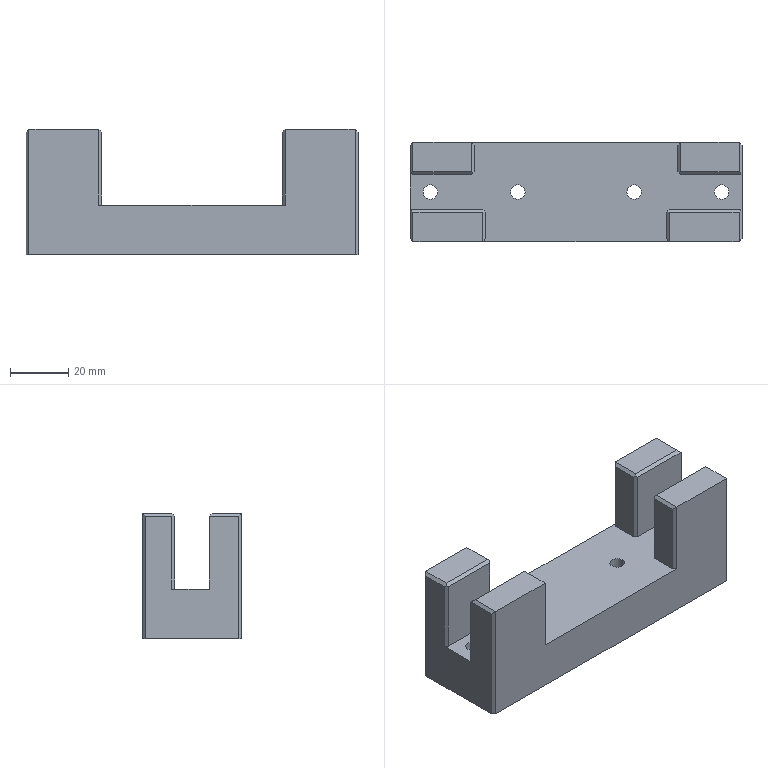Part | 1 solid | 51 faces | box 114 x 34 x 43 mm | volume 91725 mm3 | plane 43 | cylinder 8 | commonest cylinder face diameters 5 x8
STEP:
#1=CARTESIAN_POINT('',(17.5,0.,-26.));
#2=VERTEX_POINT('',#1);
#3=CARTESIAN_POINT('',(22.5,0.,-26.));
#4=VERTEX_POINT('',#3);
#5=CARTESIAN_POINT('',(20.,0.,-26.));
#6=DIRECTION('',(0.,0.,-1.));
#7=DIRECTION('',(1.,0.,0.));
#8=AXIS2_PLACEMENT_3D('',#5,#6,#7);
#9=CIRCLE('',#8,2.5);
#10=EDGE_CURVE('',#2,#4,#9,.T.);
#11=ORIENTED_EDGE('',*,*,#10,.F.);
#12=CARTESIAN_POINT('',(17.5,0.,-43.));
#13=VERTEX_POINT('',#12);
#14=CARTESIAN_POINT('',(17.5,0.,-43.));
#15=DIRECTION('',(0.,0.,-1.));
#16=VECTOR('',#15,1000.);
#17=LINE('',#14,#16);
#18=EDGE_CURVE('',#2,#13,#17,.T.);
#19=ORIENTED_EDGE('',*,*,#18,.T.);
#20=CARTESIAN_POINT('',(22.5,0.,-43.));
#21=VERTEX_POINT('',#20);
#22=CARTESIAN_POINT('',(20.,0.,-43.));
#23=DIRECTION('',(0.,0.,-1.));
#24=DIRECTION('',(1.,0.,0.));
#25=AXIS2_PLACEMENT_3D('',#22,#23,#24);
#26=CIRCLE('',#25,2.5);
#27=EDGE_CURVE('',#13,#21,#26,.T.);
#28=ORIENTED_EDGE('',*,*,#27,.T.);
#29=CARTESIAN_POINT('',(22.5,0.,-43.));
#30=DIRECTION('',(0.,0.,-1.));
#31=VECTOR('',#30,1000.);
#32=LINE('',#29,#31);
#33=EDGE_CURVE('',#4,#21,#32,.T.);
#34=ORIENTED_EDGE('',*,*,#33,.F.);
#35=EDGE_LOOP('',(#11,#19,#28,#34));
#36=FACE_BOUND('',#35,.T.);
#37=CARTESIAN_POINT('',(20.,0.,-43.));
#38=DIRECTION('',(0.,0.,-1.));
#39=DIRECTION('',(-1.,0.,0.));
#40=AXIS2_PLACEMENT_3D('',#37,#38,#39);
#41=CYLINDRICAL_SURFACE('',#40,2.5);
#42=ADVANCED_FACE('',(#36),#41,.F.);
#43=CARTESIAN_POINT('',(-22.5,0.,-26.));
#44=VERTEX_POINT('',#43);
#45=CARTESIAN_POINT('',(-17.5,0.,-26.));
#46=VERTEX_POINT('',#45);
#47=CARTESIAN_POINT('',(-20.,0.,-26.));
#48=DIRECTION('',(0.,0.,-1.));
#49=DIRECTION('',(1.,0.,0.));
#50=AXIS2_PLACEMENT_3D('',#47,#48,#49);
#51=CIRCLE('',#50,2.5);
#52=EDGE_CURVE('',#44,#46,#51,.T.);
#53=ORIENTED_EDGE('',*,*,#52,.F.);
#54=CARTESIAN_POINT('',(-22.5,0.,-43.));
#55=VERTEX_POINT('',#54);
#56=CARTESIAN_POINT('',(-22.5,0.,-43.));
#57=DIRECTION('',(0.,0.,-1.));
#58=VECTOR('',#57,1000.);
#59=LINE('',#56,#58);
#60=EDGE_CURVE('',#44,#55,#59,.T.);
#61=ORIENTED_EDGE('',*,*,#60,.T.);
#62=CARTESIAN_POINT('',(-17.5,0.,-43.));
#63=VERTEX_POINT('',#62);
#64=CARTESIAN_POINT('',(-20.,0.,-43.));
#65=DIRECTION('',(0.,0.,-1.));
#66=DIRECTION('',(1.,0.,0.));
#67=AXIS2_PLACEMENT_3D('',#64,#65,#66);
#68=CIRCLE('',#67,2.5);
#69=EDGE_CURVE('',#55,#63,#68,.T.);
#70=ORIENTED_EDGE('',*,*,#69,.T.);
#71=CARTESIAN_POINT('',(-17.5,0.,-43.));
#72=DIRECTION('',(0.,0.,-1.));
#73=VECTOR('',#72,1000.);
#74=LINE('',#71,#73);
#75=EDGE_CURVE('',#46,#63,#74,.T.);
#76=ORIENTED_EDGE('',*,*,#75,.F.);
#77=EDGE_LOOP('',(#53,#61,#70,#76));
#78=FACE_BOUND('',#77,.T.);
#79=CARTESIAN_POINT('',(-20.,0.,-43.));
#80=DIRECTION('',(0.,0.,-1.));
#81=DIRECTION('',(-1.,0.,0.));
#82=AXIS2_PLACEMENT_3D('',#79,#80,#81);
#83=CYLINDRICAL_SURFACE('',#82,2.5);
#84=ADVANCED_FACE('',(#78),#83,.F.);
#85=CARTESIAN_POINT('',(-52.5,0.,-26.));
#86=VERTEX_POINT('',#85);
#87=CARTESIAN_POINT('',(-47.5,0.,-26.));
#88=VERTEX_POINT('',#87);
#89=CARTESIAN_POINT('',(-50.,0.,-26.));
#90=DIRECTION('',(0.,0.,-1.));
#91=DIRECTION('',(1.,0.,0.));
#92=AXIS2_PLACEMENT_3D('',#89,#90,#91);
#93=CIRCLE('',#92,2.5);
#94=EDGE_CURVE('',#86,#88,#93,.T.);
#95=ORIENTED_EDGE('',*,*,#94,.F.);
#96=CARTESIAN_POINT('',(-52.5,0.,-43.));
#97=VERTEX_POINT('',#96);
#98=CARTESIAN_POINT('',(-52.5,0.,-43.));
#99=DIRECTION('',(0.,0.,-1.));
#100=VECTOR('',#99,1000.);
#101=LINE('',#98,#100);
#102=EDGE_CURVE('',#86,#97,#101,.T.);
#103=ORIENTED_EDGE('',*,*,#102,.T.);
#104=CARTESIAN_POINT('',(-47.5,0.,-43.));
#105=VERTEX_POINT('',#104);
#106=CARTESIAN_POINT('',(-50.,0.,-43.));
#107=DIRECTION('',(0.,0.,-1.));
#108=DIRECTION('',(1.,0.,0.));
#109=AXIS2_PLACEMENT_3D('',#106,#107,#108);
#110=CIRCLE('',#109,2.5);
#111=EDGE_CURVE('',#97,#105,#110,.T.);
#112=ORIENTED_EDGE('',*,*,#111,.T.);
#113=CARTESIAN_POINT('',(-47.5,0.,-43.));
#114=DIRECTION('',(0.,0.,-1.));
#115=VECTOR('',#114,1000.);
#116=LINE('',#113,#115);
#117=EDGE_CURVE('',#88,#105,#116,.T.);
#118=ORIENTED_EDGE('',*,*,#117,.F.);
#119=EDGE_LOOP('',(#95,#103,#112,#118));
#120=FACE_BOUND('',#119,.T.);
#121=CARTESIAN_POINT('',(-50.,0.,-43.));
#122=DIRECTION('',(0.,0.,-1.));
#123=DIRECTION('',(-1.,0.,0.));
#124=AXIS2_PLACEMENT_3D('',#121,#122,#123);
#125=CYLINDRICAL_SURFACE('',#124,2.5);
#126=ADVANCED_FACE('',(#120),#125,.F.);
#127=CARTESIAN_POINT('',(47.5,0.,-26.));
#128=VERTEX_POINT('',#127);
#129=CARTESIAN_POINT('',(52.5,0.,-26.));
#130=VERTEX_POINT('',#129);
#131=CARTESIAN_POINT('',(50.,0.,-26.));
#132=DIRECTION('',(0.,0.,-1.));
#133=DIRECTION('',(1.,0.,0.));
#134=AXIS2_PLACEMENT_3D('',#131,#132,#133);
#135=CIRCLE('',#134,2.5);
#136=EDGE_CURVE('',#128,#130,#135,.T.);
#137=ORIENTED_EDGE('',*,*,#136,.F.);
#138=CARTESIAN_POINT('',(47.5,0.,-43.));
#139=VERTEX_POINT('',#138);
#140=CARTESIAN_POINT('',(47.5,0.,-43.));
#141=DIRECTION('',(0.,0.,-1.));
#142=VECTOR('',#141,1000.);
#143=LINE('',#140,#142);
#144=EDGE_CURVE('',#128,#139,#143,.T.);
#145=ORIENTED_EDGE('',*,*,#144,.T.);
#146=CARTESIAN_POINT('',(52.5,0.,-43.));
#147=VERTEX_POINT('',#146);
#148=CARTESIAN_POINT('',(50.,0.,-43.));
#149=DIRECTION('',(0.,0.,-1.));
#150=DIRECTION('',(1.,0.,0.));
#151=AXIS2_PLACEMENT_3D('',#148,#149,#150);
#152=CIRCLE('',#151,2.5);
#153=EDGE_CURVE('',#139,#147,#152,.T.);
#154=ORIENTED_EDGE('',*,*,#153,.T.);
#155=CARTESIAN_POINT('',(52.5,0.,-43.));
#156=DIRECTION('',(0.,0.,-1.));
#157=VECTOR('',#156,1000.);
#158=LINE('',#155,#157);
#159=EDGE_CURVE('',#130,#147,#158,.T.);
#160=ORIENTED_EDGE('',*,*,#159,.F.);
#161=EDGE_LOOP('',(#137,#145,#154,#160));
#162=FACE_BOUND('',#161,.T.);
#163=CARTESIAN_POINT('',(50.,0.,-43.));
#164=DIRECTION('',(0.,0.,-1.));
#165=DIRECTION('',(-1.,0.,0.));
#166=AXIS2_PLACEMENT_3D('',#163,#164,#165);
#167=CYLINDRICAL_SURFACE('',#166,2.5);
#168=ADVANCED_FACE('',(#162),#167,.F.);
#169=CARTESIAN_POINT('',(36.,6.,-26.));
#170=VERTEX_POINT('',#169);
#171=CARTESIAN_POINT('',(57.,6.,-26.));
#172=VERTEX_POINT('',#171);
#173=CARTESIAN_POINT('',(57.,6.,-26.));
#174=DIRECTION('',(1.,0.,0.));
#175=VECTOR('',#174,1000.);
#176=LINE('',#173,#175);
#177=EDGE_CURVE('',#170,#172,#176,.T.);
#178=ORIENTED_EDGE('',*,*,#177,.F.);
#179=CARTESIAN_POINT('',(35.,7.,-26.));
#180=VERTEX_POINT('',#179);
#181=CARTESIAN_POINT('',(21.,21.,-26.));
#182=DIRECTION('',(-0.7071,0.7071,0.));
#183=VECTOR('',#182,1000.);
#184=LINE('',#181,#183);
#185=EDGE_CURVE('',#170,#180,#184,.T.);
#186=ORIENTED_EDGE('',*,*,#185,.T.);
#187=CARTESIAN_POINT('',(35.,16.,-26.));
#188=VERTEX_POINT('',#187);
#189=CARTESIAN_POINT('',(35.,5.,-26.));
#190=DIRECTION('',(0.,1.,0.));
#191=VECTOR('',#190,1000.);
#192=LINE('',#189,#191);
#193=EDGE_CURVE('',#180,#188,#192,.T.);
#194=ORIENTED_EDGE('',*,*,#193,.T.);
#195=CARTESIAN_POINT('',(36.,17.,-26.));
#196=VERTEX_POINT('',#195);
#197=CARTESIAN_POINT('',(9.5,-9.5,-26.));
#198=DIRECTION('',(0.7071,0.7071,0.));
#199=VECTOR('',#198,1000.);
#200=LINE('',#197,#199);
#201=EDGE_CURVE('',#188,#196,#200,.T.);
#202=ORIENTED_EDGE('',*,*,#201,.T.);
#203=CARTESIAN_POINT('',(-36.,17.,-26.));
#204=VERTEX_POINT('',#203);
#205=CARTESIAN_POINT('',(-57.,17.,-26.));
#206=DIRECTION('',(1.,0.,0.));
#207=VECTOR('',#206,1000.);
#208=LINE('',#205,#207);
#209=EDGE_CURVE('',#204,#196,#208,.T.);
#210=ORIENTED_EDGE('',*,*,#209,.F.);
#211=CARTESIAN_POINT('',(-35.,16.,-26.));
#212=VERTEX_POINT('',#211);
#213=CARTESIAN_POINT('',(-9.5,-9.5,-26.));
#214=DIRECTION('',(0.7071,-0.7071,0.));
#215=VECTOR('',#214,1000.);
#216=LINE('',#213,#215);
#217=EDGE_CURVE('',#204,#212,#216,.T.);
#218=ORIENTED_EDGE('',*,*,#217,.T.);
#219=CARTESIAN_POINT('',(-35.,7.,-26.));
#220=VERTEX_POINT('',#219);
#221=CARTESIAN_POINT('',(-35.,5.,-26.));
#222=DIRECTION('',(0.,1.,0.));
#223=VECTOR('',#222,1000.);
#224=LINE('',#221,#223);
#225=EDGE_CURVE('',#220,#212,#224,.T.);
#226=ORIENTED_EDGE('',*,*,#225,.F.);
#227=CARTESIAN_POINT('',(-36.,6.,-26.));
#228=VERTEX_POINT('',#227);
#229=CARTESIAN_POINT('',(-21.,21.,-26.));
#230=DIRECTION('',(-0.7071,-0.7071,0.));
#231=VECTOR('',#230,1000.);
#232=LINE('',#229,#231);
#233=EDGE_CURVE('',#220,#228,#232,.T.);
#234=ORIENTED_EDGE('',*,*,#233,.T.);
#235=CARTESIAN_POINT('',(-56.,6.,-26.));
#236=VERTEX_POINT('',#235);
#237=CARTESIAN_POINT('',(-57.,6.,-26.));
#238=DIRECTION('',(1.,0.,0.));
#239=VECTOR('',#238,1000.);
#240=LINE('',#237,#239);
#241=EDGE_CURVE('',#236,#228,#240,.T.);
#242=ORIENTED_EDGE('',*,*,#241,.F.);
#243=CARTESIAN_POINT('',(-57.,7.,-26.));
#244=VERTEX_POINT('',#243);
#245=CARTESIAN_POINT('',(-25.,-25.,-26.));
#246=DIRECTION('',(-0.7071,0.7071,0.));
#247=VECTOR('',#246,1000.);
#248=LINE('',#245,#247);
#249=EDGE_CURVE('',#236,#244,#248,.T.);
#250=ORIENTED_EDGE('',*,*,#249,.T.);
#251=CARTESIAN_POINT('',(-57.,-6.,-26.));
#252=VERTEX_POINT('',#251);
#253=CARTESIAN_POINT('',(-57.,-17.,-26.));
#254=DIRECTION('',(0.,1.,0.));
#255=VECTOR('',#254,1000.);
#256=LINE('',#253,#255);
#257=EDGE_CURVE('',#252,#244,#256,.T.);
#258=ORIENTED_EDGE('',*,*,#257,.F.);
#259=CARTESIAN_POINT('',(-32.,-6.,-26.));
#260=VERTEX_POINT('',#259);
#261=CARTESIAN_POINT('',(-57.,-6.,-26.));
#262=DIRECTION('',(-1.,0.,0.));
#263=VECTOR('',#262,1000.);
#264=LINE('',#261,#263);
#265=EDGE_CURVE('',#260,#252,#264,.T.);
#266=ORIENTED_EDGE('',*,*,#265,.F.);
#267=CARTESIAN_POINT('',(-31.,-7.,-26.));
#268=VERTEX_POINT('',#267);
#269=CARTESIAN_POINT('',(-19.,-19.,-26.));
#270=DIRECTION('',(0.7071,-0.7071,0.));
#271=VECTOR('',#270,1000.);
#272=LINE('',#269,#271);
#273=EDGE_CURVE('',#260,#268,#272,.T.);
#274=ORIENTED_EDGE('',*,*,#273,.T.);
#275=CARTESIAN_POINT('',(-31.,-16.,-26.));
#276=VERTEX_POINT('',#275);
#277=CARTESIAN_POINT('',(-31.,-17.,-26.));
#278=DIRECTION('',(0.,1.,0.));
#279=VECTOR('',#278,1000.);
#280=LINE('',#277,#279);
#281=EDGE_CURVE('',#276,#268,#280,.T.);
#282=ORIENTED_EDGE('',*,*,#281,.F.);
#283=CARTESIAN_POINT('',(-32.,-17.,-26.));
#284=VERTEX_POINT('',#283);
#285=CARTESIAN_POINT('',(-7.5,7.5,-26.));
#286=DIRECTION('',(-0.7071,-0.7071,0.));
#287=VECTOR('',#286,1000.);
#288=LINE('',#285,#287);
#289=EDGE_CURVE('',#276,#284,#288,.T.);
#290=ORIENTED_EDGE('',*,*,#289,.T.);
#291=CARTESIAN_POINT('',(32.,-17.,-26.));
#292=VERTEX_POINT('',#291);
#293=CARTESIAN_POINT('',(-57.,-17.,-26.));
#294=DIRECTION('',(-1.,0.,0.));
#295=VECTOR('',#294,1000.);
#296=LINE('',#293,#295);
#297=EDGE_CURVE('',#292,#284,#296,.T.);
#298=ORIENTED_EDGE('',*,*,#297,.F.);
#299=CARTESIAN_POINT('',(31.,-16.,-26.));
#300=VERTEX_POINT('',#299);
#301=CARTESIAN_POINT('',(7.5,7.5,-26.));
#302=DIRECTION('',(-0.7071,0.7071,0.));
#303=VECTOR('',#302,1000.);
#304=LINE('',#301,#303);
#305=EDGE_CURVE('',#292,#300,#304,.T.);
#306=ORIENTED_EDGE('',*,*,#305,.T.);
#307=CARTESIAN_POINT('',(31.,-7.,-26.));
#308=VERTEX_POINT('',#307);
#309=CARTESIAN_POINT('',(31.,-17.,-26.));
#310=DIRECTION('',(0.,-1.,0.));
#311=VECTOR('',#310,1000.);
#312=LINE('',#309,#311);
#313=EDGE_CURVE('',#308,#300,#312,.T.);
#314=ORIENTED_EDGE('',*,*,#313,.F.);
#315=CARTESIAN_POINT('',(32.,-6.,-26.));
#316=VERTEX_POINT('',#315);
#317=CARTESIAN_POINT('',(19.,-19.,-26.));
#318=DIRECTION('',(0.7071,0.7071,0.));
#319=VECTOR('',#318,1000.);
#320=LINE('',#317,#319);
#321=EDGE_CURVE('',#308,#316,#320,.T.);
#322=ORIENTED_EDGE('',*,*,#321,.T.);
#323=CARTESIAN_POINT('',(57.,-6.,-26.));
#324=VERTEX_POINT('',#323);
#325=CARTESIAN_POINT('',(57.,-6.,-26.));
#326=DIRECTION('',(-1.,0.,0.));
#327=VECTOR('',#326,1000.);
#328=LINE('',#325,#327);
#329=EDGE_CURVE('',#324,#316,#328,.T.);
#330=ORIENTED_EDGE('',*,*,#329,.F.);
#331=CARTESIAN_POINT('',(57.,-17.,-26.));
#332=DIRECTION('',(0.,-1.,0.));
#333=VECTOR('',#332,1000.);
#334=LINE('',#331,#333);
#335=EDGE_CURVE('',#172,#324,#334,.T.);
#336=ORIENTED_EDGE('',*,*,#335,.F.);
#337=EDGE_LOOP('',(#178,#186,#194,#202,#210,#218,#226,#234,#242,#250,#258,#266,#274,#282,#290,#298,#306,#314,#322,#330,#336));
#338=FACE_BOUND('',#337,.T.);
#339=CARTESIAN_POINT('',(20.,0.,-26.));
#340=DIRECTION('',(0.,0.,-1.));
#341=DIRECTION('',(1.,0.,0.));
#342=AXIS2_PLACEMENT_3D('',#339,#340,#341);
#343=CIRCLE('',#342,2.5);
#344=EDGE_CURVE('',#4,#2,#343,.T.);
#345=ORIENTED_EDGE('',*,*,#344,.T.);
#346=ORIENTED_EDGE('',*,*,#10,.T.);
#347=EDGE_LOOP('',(#345,#346));
#348=FACE_BOUND('',#347,.T.);
#349=CARTESIAN_POINT('',(-20.,0.,-26.));
#350=DIRECTION('',(0.,0.,-1.));
#351=DIRECTION('',(1.,0.,0.));
#352=AXIS2_PLACEMENT_3D('',#349,#350,#351);
#353=CIRCLE('',#352,2.5);
#354=EDGE_CURVE('',#46,#44,#353,.T.);
#355=ORIENTED_EDGE('',*,*,#354,.T.);
#356=ORIENTED_EDGE('',*,*,#52,.T.);
#357=EDGE_LOOP('',(#355,#356));
#358=FACE_BOUND('',#357,.T.);
#359=CARTESIAN_POINT('',(-50.,0.,-26.));
#360=DIRECTION('',(0.,0.,-1.));
#361=DIRECTION('',(1.,0.,0.));
#362=AXIS2_PLACEMENT_3D('',#359,#360,#361);
#363=CIRCLE('',#362,2.5);
#364=EDGE_CURVE('',#88,#86,#363,.T.);
#365=ORIENTED_EDGE('',*,*,#364,.T.);
#366=ORIENTED_EDGE('',*,*,#94,.T.);
#367=EDGE_LOOP('',(#365,#366));
#368=FACE_BOUND('',#367,.T.);
#369=CARTESIAN_POINT('',(50.,0.,-26.));
#370=DIRECTION('',(0.,0.,-1.));
#371=DIRECTION('',(1.,0.,0.));
#372=AXIS2_PLACEMENT_3D('',#369,#370,#371);
#373=CIRCLE('',#372,2.5);
#374=EDGE_CURVE('',#130,#128,#373,.T.);
#375=ORIENTED_EDGE('',*,*,#374,.T.);
#376=ORIENTED_EDGE('',*,*,#136,.T.);
#377=EDGE_LOOP('',(#375,#376));
#378=FACE_BOUND('',#377,.T.);
#379=CARTESIAN_POINT('',(0.,0.,-26.));
#380=DIRECTION('',(0.,0.,-1.));
#381=DIRECTION('',(-1.,0.,0.));
#382=AXIS2_PLACEMENT_3D('',#379,#380,#381);
#383=PLANE('',#382);
#384=ADVANCED_FACE('',(#338,#348,#358,#368,#378),#383,.F.);
#385=CARTESIAN_POINT('',(57.,16.,-43.));
#386=VERTEX_POINT('',#385);
#387=CARTESIAN_POINT('',(57.,-16.,-43.));
#388=VERTEX_POINT('',#387);
#389=CARTESIAN_POINT('',(57.,-17.,-43.));
#390=DIRECTION('',(0.,-1.,0.));
#391=VECTOR('',#390,1000.);
#392=LINE('',#389,#391);
#393=EDGE_CURVE('',#386,#388,#392,.T.);
#394=ORIENTED_EDGE('',*,*,#393,.F.);
#395=CARTESIAN_POINT('',(57.,16.,-1.));
#396=VERTEX_POINT('',#395);
#397=CARTESIAN_POINT('',(57.,16.,-43.));
#398=DIRECTION('',(0.,0.,1.));
#399=VECTOR('',#398,1000.);
#400=LINE('',#397,#399);
#401=EDGE_CURVE('',#386,#396,#400,.T.);
#402=ORIENTED_EDGE('',*,*,#401,.T.);
#403=CARTESIAN_POINT('',(57.,6.,-1.));
#404=VERTEX_POINT('',#403);
#405=CARTESIAN_POINT('',(57.,7.,-1.));
#406=DIRECTION('',(0.,-1.,0.));
#407=VECTOR('',#406,1000.);
#408=LINE('',#405,#407);
#409=EDGE_CURVE('',#396,#404,#408,.T.);
#410=ORIENTED_EDGE('',*,*,#409,.T.);
#411=CARTESIAN_POINT('',(57.,6.,0.));
#412=DIRECTION('',(0.,0.,-1.));
#413=VECTOR('',#412,1000.);
#414=LINE('',#411,#413);
#415=EDGE_CURVE('',#404,#172,#414,.T.);
#416=ORIENTED_EDGE('',*,*,#415,.T.);
#417=ORIENTED_EDGE('',*,*,#335,.T.);
#418=CARTESIAN_POINT('',(57.,-6.,-1.));
#419=VERTEX_POINT('',#418);
#420=CARTESIAN_POINT('',(57.,-6.,0.));
#421=DIRECTION('',(0.,0.,-1.));
#422=VECTOR('',#421,1000.);
#423=LINE('',#420,#422);
#424=EDGE_CURVE('',#419,#324,#423,.T.);
#425=ORIENTED_EDGE('',*,*,#424,.F.);
#426=CARTESIAN_POINT('',(57.,-16.,-1.));
#427=VERTEX_POINT('',#426);
#428=CARTESIAN_POINT('',(57.,-17.,-1.));
#429=DIRECTION('',(0.,-1.,0.));
#430=VECTOR('',#429,1000.);
#431=LINE('',#428,#430);
#432=EDGE_CURVE('',#419,#427,#431,.T.);
#433=ORIENTED_EDGE('',*,*,#432,.T.);
#434=CARTESIAN_POINT('',(57.,-16.,-43.));
#435=DIRECTION('',(0.,0.,-1.));
#436=VECTOR('',#435,1000.);
#437=LINE('',#434,#436);
#438=EDGE_CURVE('',#427,#388,#437,.T.);
#439=ORIENTED_EDGE('',*,*,#438,.T.);
#440=EDGE_LOOP('',(#394,#402,#410,#416,#417,#425,#433,#439));
#441=FACE_BOUND('',#440,.T.);
#442=CARTESIAN_POINT('',(57.,-17.,-43.));
#443=DIRECTION('',(-1.,0.,0.));
#444=DIRECTION('',(0.,-1.,0.));
#445=AXIS2_PLACEMENT_3D('',#442,#443,#444);
#446=PLANE('',#445);
#447=ADVANCED_FACE('',(#441),#446,.F.);
#448=CARTESIAN_POINT('',(56.,-17.,-43.));
#449=VERTEX_POINT('',#448);
#450=CARTESIAN_POINT('',(-56.,-17.,-43.));
#451=VERTEX_POINT('',#450);
#452=CARTESIAN_POINT('',(-57.,-17.,-43.));
#453=DIRECTION('',(-1.,0.,0.));
#454=VECTOR('',#453,1000.);
#455=LINE('',#452,#454);
#456=EDGE_CURVE('',#449,#451,#455,.T.);
#457=ORIENTED_EDGE('',*,*,#456,.F.);
#458=CARTESIAN_POINT('',(56.,-17.,0.));
#459=VERTEX_POINT('',#458);
#460=CARTESIAN_POINT('',(56.,-17.,-43.));
#461=DIRECTION('',(0.,0.,1.));
#462=VECTOR('',#461,1000.);
#463=LINE('',#460,#462);
#464=EDGE_CURVE('',#449,#459,#463,.T.);
#465=ORIENTED_EDGE('',*,*,#464,.T.);
#466=CARTESIAN_POINT('',(32.,-17.,0.));
#467=VERTEX_POINT('',#466);
#468=CARTESIAN_POINT('',(57.,-17.,0.));
#469=DIRECTION('',(1.,0.,0.));
#470=VECTOR('',#469,1000.);
#471=LINE('',#468,#470);
#472=EDGE_CURVE('',#467,#459,#471,.T.);
#473=ORIENTED_EDGE('',*,*,#472,.F.);
#474=CARTESIAN_POINT('',(32.,-17.,-43.));
#475=DIRECTION('',(0.,0.,-1.));
#476=VECTOR('',#475,1000.);
#477=LINE('',#474,#476);
#478=EDGE_CURVE('',#467,#292,#477,.T.);
#479=ORIENTED_EDGE('',*,*,#478,.T.);
#480=ORIENTED_EDGE('',*,*,#297,.T.);
#481=CARTESIAN_POINT('',(-32.,-17.,0.));
#482=VERTEX_POINT('',#481);
#483=CARTESIAN_POINT('',(-32.,-17.,-43.));
#484=DIRECTION('',(0.,0.,1.));
#485=VECTOR('',#484,1000.);
#486=LINE('',#483,#485);
#487=EDGE_CURVE('',#284,#482,#486,.T.);
#488=ORIENTED_EDGE('',*,*,#487,.T.);
#489=CARTESIAN_POINT('',(-56.,-17.,0.));
#490=VERTEX_POINT('',#489);
#491=CARTESIAN_POINT('',(-57.,-17.,0.));
#492=DIRECTION('',(1.,0.,0.));
#493=VECTOR('',#492,1000.);
#494=LINE('',#491,#493);
#495=EDGE_CURVE('',#490,#482,#494,.T.);
#496=ORIENTED_EDGE('',*,*,#495,.F.);
#497=CARTESIAN_POINT('',(-56.,-17.,-43.));
#498=DIRECTION('',(0.,0.,-1.));
#499=VECTOR('',#498,1000.);
#500=LINE('',#497,#499);
#501=EDGE_CURVE('',#490,#451,#500,.T.);
#502=ORIENTED_EDGE('',*,*,#501,.T.);
#503=EDGE_LOOP('',(#457,#465,#473,#479,#480,#488,#496,#502));
#504=FACE_BOUND('',#503,.T.);
#505=CARTESIAN_POINT('',(-57.,-17.,-43.));
#506=DIRECTION('',(0.,1.,0.));
#507=DIRECTION('',(0.,0.,-1.));
#508=AXIS2_PLACEMENT_3D('',#505,#506,#507);
#509=PLANE('',#508);
#510=ADVANCED_FACE('',(#504),#509,.F.);
#511=CARTESIAN_POINT('',(-57.,-16.,-43.));
#512=VERTEX_POINT('',#511);
#513=CARTESIAN_POINT('',(-57.,16.,-43.));
#514=VERTEX_POINT('',#513);
#515=CARTESIAN_POINT('',(-57.,-17.,-43.));
#516=DIRECTION('',(0.,1.,0.));
#517=VECTOR('',#516,1000.);
#518=LINE('',#515,#517);
#519=EDGE_CURVE('',#512,#514,#518,.T.);
#520=ORIENTED_EDGE('',*,*,#519,.F.);
#521=CARTESIAN_POINT('',(-57.,-16.,-1.));
#522=VERTEX_POINT('',#521);
#523=CARTESIAN_POINT('',(-57.,-16.,-43.));
#524=DIRECTION('',(0.,0.,1.));
#525=VECTOR('',#524,1000.);
#526=LINE('',#523,#525);
#527=EDGE_CURVE('',#512,#522,#526,.T.);
#528=ORIENTED_EDGE('',*,*,#527,.T.);
#529=CARTESIAN_POINT('',(-57.,-6.,-1.));
#530=VERTEX_POINT('',#529);
#531=CARTESIAN_POINT('',(-57.,-7.,-1.));
#532=DIRECTION('',(0.,1.,0.));
#533=VECTOR('',#532,1000.);
#534=LINE('',#531,#533);
#535=EDGE_CURVE('',#522,#530,#534,.T.);
#536=ORIENTED_EDGE('',*,*,#535,.T.);
#537=CARTESIAN_POINT('',(-57.,-6.,0.));
#538=DIRECTION('',(0.,0.,-1.));
#539=VECTOR('',#538,1000.);
#540=LINE('',#537,#539);
#541=EDGE_CURVE('',#530,#252,#540,.T.);
#542=ORIENTED_EDGE('',*,*,#541,.T.);
#543=ORIENTED_EDGE('',*,*,#257,.T.);
#544=CARTESIAN_POINT('',(-57.,7.,-1.));
#545=VERTEX_POINT('',#544);
#546=CARTESIAN_POINT('',(-57.,7.,-43.));
#547=DIRECTION('',(0.,0.,1.));
#548=VECTOR('',#547,1000.);
#549=LINE('',#546,#548);
#550=EDGE_CURVE('',#244,#545,#549,.T.);
#551=ORIENTED_EDGE('',*,*,#550,.T.);
#552=CARTESIAN_POINT('',(-57.,16.,-1.));
#553=VERTEX_POINT('',#552);
#554=CARTESIAN_POINT('',(-57.,17.,-1.));
#555=DIRECTION('',(0.,1.,0.));
#556=VECTOR('',#555,1000.);
#557=LINE('',#554,#556);
#558=EDGE_CURVE('',#545,#553,#557,.T.);
#559=ORIENTED_EDGE('',*,*,#558,.T.);
#560=CARTESIAN_POINT('',(-57.,16.,-43.));
#561=DIRECTION('',(0.,0.,-1.));
#562=VECTOR('',#561,1000.);
#563=LINE('',#560,#562);
#564=EDGE_CURVE('',#553,#514,#563,.T.);
#565=ORIENTED_EDGE('',*,*,#564,.T.);
#566=EDGE_LOOP('',(#520,#528,#536,#542,#543,#551,#559,#565));
#567=FACE_BOUND('',#566,.T.);
#568=CARTESIAN_POINT('',(-57.,-17.,-43.));
#569=DIRECTION('',(1.,0.,0.));
#570=DIRECTION('',(0.,1.,0.));
#571=AXIS2_PLACEMENT_3D('',#568,#569,#570);
#572=PLANE('',#571);
#573=ADVANCED_FACE('',(#567),#572,.F.);
#574=CARTESIAN_POINT('',(56.,17.,0.));
#575=VERTEX_POINT('',#574);
#576=CARTESIAN_POINT('',(36.,17.,0.));
#577=VERTEX_POINT('',#576);
#578=CARTESIAN_POINT('',(57.,17.,0.));
#579=DIRECTION('',(-1.,0.,0.));
#580=VECTOR('',#579,1000.);
#581=LINE('',#578,#580);
#582=EDGE_CURVE('',#575,#577,#581,.T.);
#583=ORIENTED_EDGE('',*,*,#582,.F.);
#584=CARTESIAN_POINT('',(56.,17.,-43.));
#585=VERTEX_POINT('',#584);
#586=CARTESIAN_POINT('',(56.,17.,-43.));
#587=DIRECTION('',(0.,0.,-1.));
#588=VECTOR('',#587,1000.);
#589=LINE('',#586,#588);
#590=EDGE_CURVE('',#575,#585,#589,.T.);
#591=ORIENTED_EDGE('',*,*,#590,.T.);
#592=CARTESIAN_POINT('',(-56.,17.,-43.));
#593=VERTEX_POINT('',#592);
#594=CARTESIAN_POINT('',(-57.,17.,-43.));
#595=DIRECTION('',(1.,0.,0.));
#596=VECTOR('',#595,1000.);
#597=LINE('',#594,#596);
#598=EDGE_CURVE('',#593,#585,#597,.T.);
#599=ORIENTED_EDGE('',*,*,#598,.F.);
#600=CARTESIAN_POINT('',(-56.,17.,0.));
#601=VERTEX_POINT('',#600);
#602=CARTESIAN_POINT('',(-56.,17.,-43.));
#603=DIRECTION('',(0.,0.,1.));
#604=VECTOR('',#603,1000.);
#605=LINE('',#602,#604);
#606=EDGE_CURVE('',#593,#601,#605,.T.);
#607=ORIENTED_EDGE('',*,*,#606,.T.);
#608=CARTESIAN_POINT('',(-36.,17.,0.));
#609=VERTEX_POINT('',#608);
#610=CARTESIAN_POINT('',(-57.,17.,0.));
#611=DIRECTION('',(-1.,0.,0.));
#612=VECTOR('',#611,1000.);
#613=LINE('',#610,#612);
#614=EDGE_CURVE('',#609,#601,#613,.T.);
#615=ORIENTED_EDGE('',*,*,#614,.F.);
#616=CARTESIAN_POINT('',(-36.,17.,-43.));
#617=DIRECTION('',(0.,0.,-1.));
#618=VECTOR('',#617,1000.);
#619=LINE('',#616,#618);
#620=EDGE_CURVE('',#609,#204,#619,.T.);
#621=ORIENTED_EDGE('',*,*,#620,.T.);
#622=ORIENTED_EDGE('',*,*,#209,.T.);
#623=CARTESIAN_POINT('',(36.,17.,-43.));
#624=DIRECTION('',(0.,0.,1.));
#625=VECTOR('',#624,1000.);
#626=LINE('',#623,#625);
#627=EDGE_CURVE('',#196,#577,#626,.T.);
#628=ORIENTED_EDGE('',*,*,#627,.T.);
#629=EDGE_LOOP('',(#583,#591,#599,#607,#615,#621,#622,#628));
#630=FACE_BOUND('',#629,.T.);
#631=CARTESIAN_POINT('',(-57.,17.,-43.));
#632=DIRECTION('',(0.,-1.,0.));
#633=DIRECTION('',(0.,0.,1.));
#634=AXIS2_PLACEMENT_3D('',#631,#632,#633);
#635=PLANE('',#634);
#636=ADVANCED_FACE('',(#630),#635,.F.);
#637=CARTESIAN_POINT('',(20.,0.,-43.));
#638=DIRECTION('',(0.,0.,-1.));
#639=DIRECTION('',(1.,0.,0.));
#640=AXIS2_PLACEMENT_3D('',#637,#638,#639);
#641=CIRCLE('',#640,2.5);
#642=EDGE_CURVE('',#21,#13,#641,.T.);
#643=ORIENTED_EDGE('',*,*,#642,.F.);
#644=ORIENTED_EDGE('',*,*,#27,.F.);
#645=EDGE_LOOP('',(#643,#644));
#646=FACE_BOUND('',#645,.T.);
#647=CARTESIAN_POINT('',(-20.,0.,-43.));
#648=DIRECTION('',(0.,0.,-1.));
#649=DIRECTION('',(1.,0.,0.));
#650=AXIS2_PLACEMENT_3D('',#647,#648,#649);
#651=CIRCLE('',#650,2.5);
#652=EDGE_CURVE('',#63,#55,#651,.T.);
#653=ORIENTED_EDGE('',*,*,#652,.F.);
#654=ORIENTED_EDGE('',*,*,#69,.F.);
#655=EDGE_LOOP('',(#653,#654));
#656=FACE_BOUND('',#655,.T.);
#657=CARTESIAN_POINT('',(-50.,0.,-43.));
#658=DIRECTION('',(0.,0.,-1.));
#659=DIRECTION('',(1.,0.,0.));
#660=AXIS2_PLACEMENT_3D('',#657,#658,#659);
#661=CIRCLE('',#660,2.5);
#662=EDGE_CURVE('',#105,#97,#661,.T.);
#663=ORIENTED_EDGE('',*,*,#662,.F.);
#664=ORIENTED_EDGE('',*,*,#111,.F.);
#665=EDGE_LOOP('',(#663,#664));
#666=FACE_BOUND('',#665,.T.);
#667=CARTESIAN_POINT('',(50.,0.,-43.));
#668=DIRECTION('',(0.,0.,-1.));
#669=DIRECTION('',(1.,0.,0.));
#670=AXIS2_PLACEMENT_3D('',#667,#668,#669);
#671=CIRCLE('',#670,2.5);
#672=EDGE_CURVE('',#147,#139,#671,.T.);
#673=ORIENTED_EDGE('',*,*,#672,.F.);
#674=ORIENTED_EDGE('',*,*,#153,.F.);
#675=EDGE_LOOP('',(#673,#674));
#676=FACE_BOUND('',#675,.T.);
#677=ORIENTED_EDGE('',*,*,#598,.T.);
#678=CARTESIAN_POINT('',(36.5,36.5,-43.));
#679=DIRECTION('',(0.7071,-0.7071,0.));
#680=VECTOR('',#679,1000.);
#681=LINE('',#678,#680);
#682=EDGE_CURVE('',#585,#386,#681,.T.);
#683=ORIENTED_EDGE('',*,*,#682,.T.);
#684=ORIENTED_EDGE('',*,*,#393,.T.);
#685=CARTESIAN_POINT('',(36.5,-36.5,-43.));
#686=DIRECTION('',(-0.7071,-0.7071,0.));
#687=VECTOR('',#686,1000.);
#688=LINE('',#685,#687);
#689=EDGE_CURVE('',#388,#449,#688,.T.);
#690=ORIENTED_EDGE('',*,*,#689,.T.);
#691=ORIENTED_EDGE('',*,*,#456,.T.);
#692=CARTESIAN_POINT('',(-36.5,-36.5,-43.));
#693=DIRECTION('',(-0.7071,0.7071,0.));
#694=VECTOR('',#693,1000.);
#695=LINE('',#692,#694);
#696=EDGE_CURVE('',#451,#512,#695,.T.);
#697=ORIENTED_EDGE('',*,*,#696,.T.);
#698=ORIENTED_EDGE('',*,*,#519,.T.);
#699=CARTESIAN_POINT('',(-36.5,36.5,-43.));
#700=DIRECTION('',(0.7071,0.7071,0.));
#701=VECTOR('',#700,1000.);
#702=LINE('',#699,#701);
#703=EDGE_CURVE('',#514,#593,#702,.T.);
#704=ORIENTED_EDGE('',*,*,#703,.T.);
#705=EDGE_LOOP('',(#677,#683,#684,#690,#691,#697,#698,#704));
#706=FACE_BOUND('',#705,.T.);
#707=CARTESIAN_POINT('',(0.,0.,-43.));
#708=DIRECTION('',(0.,0.,-1.));
#709=DIRECTION('',(-1.,0.,0.));
#710=AXIS2_PLACEMENT_3D('',#707,#708,#709);
#711=PLANE('',#710);
#712=ADVANCED_FACE('',(#646,#656,#666,#676,#706),#711,.T.);
#713=ORIENTED_EDGE('',*,*,#329,.T.);
#714=CARTESIAN_POINT('',(32.,-6.,-1.));
#715=VERTEX_POINT('',#714);
#716=CARTESIAN_POINT('',(32.,-6.,0.));
#717=DIRECTION('',(0.,0.,1.));
#718=VECTOR('',#717,1000.);
#719=LINE('',#716,#718);
#720=EDGE_CURVE('',#316,#715,#719,.T.);
#721=ORIENTED_EDGE('',*,*,#720,.T.);
#722=CARTESIAN_POINT('',(57.,-6.,-1.));
#723=DIRECTION('',(1.,0.,0.));
#724=VECTOR('',#723,1000.);
#725=LINE('',#722,#724);
#726=EDGE_CURVE('',#715,#419,#725,.T.);
#727=ORIENTED_EDGE('',*,*,#726,.T.);
#728=ORIENTED_EDGE('',*,*,#424,.T.);
#729=EDGE_LOOP('',(#713,#721,#727,#728));
#730=FACE_BOUND('',#729,.T.);
#731=CARTESIAN_POINT('',(57.,-6.,0.));
#732=DIRECTION('',(0.,-1.,0.));
#733=DIRECTION('',(1.,0.,0.));
#734=AXIS2_PLACEMENT_3D('',#731,#732,#733);
#735=PLANE('',#734);
#736=ADVANCED_FACE('',(#730),#735,.F.);
#737=ORIENTED_EDGE('',*,*,#313,.T.);
#738=CARTESIAN_POINT('',(31.,-16.,-1.));
#739=VERTEX_POINT('',#738);
#740=CARTESIAN_POINT('',(31.,-16.,0.));
#741=DIRECTION('',(0.,0.,1.));
#742=VECTOR('',#741,1000.);
#743=LINE('',#740,#742);
#744=EDGE_CURVE('',#300,#739,#743,.T.);
#745=ORIENTED_EDGE('',*,*,#744,.T.);
#746=CARTESIAN_POINT('',(31.,-7.,-1.));
#747=VERTEX_POINT('',#746);
#748=CARTESIAN_POINT('',(31.,-7.,-1.));
#749=DIRECTION('',(0.,1.,0.));
#750=VECTOR('',#749,1000.);
#751=LINE('',#748,#750);
#752=EDGE_CURVE('',#739,#747,#751,.T.);
#753=ORIENTED_EDGE('',*,*,#752,.T.);
#754=CARTESIAN_POINT('',(31.,-7.,0.));
#755=DIRECTION('',(0.,0.,-1.));
#756=VECTOR('',#755,1000.);
#757=LINE('',#754,#756);
#758=EDGE_CURVE('',#747,#308,#757,.T.);
#759=ORIENTED_EDGE('',*,*,#758,.T.);
#760=EDGE_LOOP('',(#737,#745,#753,#759));
#761=FACE_BOUND('',#760,.T.);
#762=CARTESIAN_POINT('',(31.,-17.,0.));
#763=DIRECTION('',(1.,0.,0.));
#764=DIRECTION('',(0.,1.,0.));
#765=AXIS2_PLACEMENT_3D('',#762,#763,#764);
#766=PLANE('',#765);
#767=ADVANCED_FACE('',(#761),#766,.F.);
#768=CARTESIAN_POINT('',(56.,-7.,0.));
#769=VERTEX_POINT('',#768);
#770=CARTESIAN_POINT('',(32.,-7.,0.));
#771=VERTEX_POINT('',#770);
#772=CARTESIAN_POINT('',(31.,-7.,0.));
#773=DIRECTION('',(-1.,0.,0.));
#774=VECTOR('',#773,1000.);
#775=LINE('',#772,#774);
#776=EDGE_CURVE('',#769,#771,#775,.T.);
#777=ORIENTED_EDGE('',*,*,#776,.T.);
#778=CARTESIAN_POINT('',(32.,-17.,0.));
#779=DIRECTION('',(0.,-1.,0.));
#780=VECTOR('',#779,1000.);
#781=LINE('',#778,#780);
#782=EDGE_CURVE('',#771,#467,#781,.T.);
#783=ORIENTED_EDGE('',*,*,#782,.T.);
#784=ORIENTED_EDGE('',*,*,#472,.T.);
#785=CARTESIAN_POINT('',(56.,-7.,0.));
#786=DIRECTION('',(0.,1.,0.));
#787=VECTOR('',#786,1000.);
#788=LINE('',#785,#787);
#789=EDGE_CURVE('',#459,#769,#788,.T.);
#790=ORIENTED_EDGE('',*,*,#789,.T.);
#791=EDGE_LOOP('',(#777,#783,#784,#790));
#792=FACE_BOUND('',#791,.T.);
#793=CARTESIAN_POINT('',(0.,0.,0.));
#794=DIRECTION('',(0.,0.,1.));
#795=DIRECTION('',(1.,0.,0.));
#796=AXIS2_PLACEMENT_3D('',#793,#794,#795);
#797=PLANE('',#796);
#798=ADVANCED_FACE('',(#792),#797,.T.);
#799=ORIENTED_EDGE('',*,*,#281,.T.);
#800=CARTESIAN_POINT('',(-31.,-7.,-1.));
#801=VERTEX_POINT('',#800);
#802=CARTESIAN_POINT('',(-31.,-7.,0.));
#803=DIRECTION('',(0.,0.,1.));
#804=VECTOR('',#803,1000.);
#805=LINE('',#802,#804);
#806=EDGE_CURVE('',#268,#801,#805,.T.);
#807=ORIENTED_EDGE('',*,*,#806,.T.);
#808=CARTESIAN_POINT('',(-31.,-16.,-1.));
#809=VERTEX_POINT('',#808);
#810=CARTESIAN_POINT('',(-31.,-17.,-1.));
#811=DIRECTION('',(0.,-1.,0.));
#812=VECTOR('',#811,1000.);
#813=LINE('',#810,#812);
#814=EDGE_CURVE('',#801,#809,#813,.T.);
#815=ORIENTED_EDGE('',*,*,#814,.T.);
#816=CARTESIAN_POINT('',(-31.,-16.,0.));
#817=DIRECTION('',(0.,0.,-1.));
#818=VECTOR('',#817,1000.);
#819=LINE('',#816,#818);
#820=EDGE_CURVE('',#809,#276,#819,.T.);
#821=ORIENTED_EDGE('',*,*,#820,.T.);
#822=EDGE_LOOP('',(#799,#807,#815,#821));
#823=FACE_BOUND('',#822,.T.);
#824=CARTESIAN_POINT('',(-31.,-17.,0.));
#825=DIRECTION('',(-1.,0.,0.));
#826=DIRECTION('',(0.,-1.,0.));
#827=AXIS2_PLACEMENT_3D('',#824,#825,#826);
#828=PLANE('',#827);
#829=ADVANCED_FACE('',(#823),#828,.F.);
#830=CARTESIAN_POINT('',(-32.,-6.,-1.));
#831=VERTEX_POINT('',#830);
#832=CARTESIAN_POINT('',(-31.,-6.,-1.));
#833=DIRECTION('',(1.,0.,0.));
#834=VECTOR('',#833,1000.);
#835=LINE('',#832,#834);
#836=EDGE_CURVE('',#530,#831,#835,.T.);
#837=ORIENTED_EDGE('',*,*,#836,.T.);
#838=CARTESIAN_POINT('',(-32.,-6.,0.));
#839=DIRECTION('',(0.,0.,-1.));
#840=VECTOR('',#839,1000.);
#841=LINE('',#838,#840);
#842=EDGE_CURVE('',#831,#260,#841,.T.);
#843=ORIENTED_EDGE('',*,*,#842,.T.);
#844=ORIENTED_EDGE('',*,*,#265,.T.);
#845=ORIENTED_EDGE('',*,*,#541,.F.);
#846=EDGE_LOOP('',(#837,#843,#844,#845));
#847=FACE_BOUND('',#846,.T.);
#848=CARTESIAN_POINT('',(-57.,-6.,0.));
#849=DIRECTION('',(0.,-1.,0.));
#850=DIRECTION('',(1.,0.,0.));
#851=AXIS2_PLACEMENT_3D('',#848,#849,#850);
#852=PLANE('',#851);
#853=ADVANCED_FACE('',(#847),#852,.F.);
#854=CARTESIAN_POINT('',(-32.,-7.,0.));
#855=VERTEX_POINT('',#854);
#856=CARTESIAN_POINT('',(-56.,-7.,0.));
#857=VERTEX_POINT('',#856);
#858=CARTESIAN_POINT('',(-57.,-7.,0.));
#859=DIRECTION('',(-1.,0.,0.));
#860=VECTOR('',#859,1000.);
#861=LINE('',#858,#860);
#862=EDGE_CURVE('',#855,#857,#861,.T.);
#863=ORIENTED_EDGE('',*,*,#862,.T.);
#864=CARTESIAN_POINT('',(-56.,-17.,0.));
#865=DIRECTION('',(0.,-1.,0.));
#866=VECTOR('',#865,1000.);
#867=LINE('',#864,#866);
#868=EDGE_CURVE('',#857,#490,#867,.T.);
#869=ORIENTED_EDGE('',*,*,#868,.T.);
#870=ORIENTED_EDGE('',*,*,#495,.T.);
#871=CARTESIAN_POINT('',(-32.,-7.,0.));
#872=DIRECTION('',(0.,1.,0.));
#873=VECTOR('',#872,1000.);
#874=LINE('',#871,#873);
#875=EDGE_CURVE('',#482,#855,#874,.T.);
#876=ORIENTED_EDGE('',*,*,#875,.T.);
#877=EDGE_LOOP('',(#863,#869,#870,#876));
#878=FACE_BOUND('',#877,.T.);
#879=CARTESIAN_POINT('',(0.,0.,0.));
#880=DIRECTION('',(0.,0.,1.));
#881=DIRECTION('',(1.,0.,0.));
#882=AXIS2_PLACEMENT_3D('',#879,#880,#881);
#883=PLANE('',#882);
#884=ADVANCED_FACE('',(#878),#883,.T.);
#885=CARTESIAN_POINT('',(-36.,6.,-1.));
#886=VERTEX_POINT('',#885);
#887=CARTESIAN_POINT('',(-56.,6.,-1.));
#888=VERTEX_POINT('',#887);
#889=CARTESIAN_POINT('',(-57.,6.,-1.));
#890=DIRECTION('',(-1.,0.,0.));
#891=VECTOR('',#890,1000.);
#892=LINE('',#889,#891);
#893=EDGE_CURVE('',#886,#888,#892,.T.);
#894=ORIENTED_EDGE('',*,*,#893,.T.);
#895=CARTESIAN_POINT('',(-56.,6.,0.));
#896=DIRECTION('',(0.,0.,-1.));
#897=VECTOR('',#896,1000.);
#898=LINE('',#895,#897);
#899=EDGE_CURVE('',#888,#236,#898,.T.);
#900=ORIENTED_EDGE('',*,*,#899,.T.);
#901=ORIENTED_EDGE('',*,*,#241,.T.);
#902=CARTESIAN_POINT('',(-36.,6.,0.));
#903=DIRECTION('',(0.,0.,1.));
#904=VECTOR('',#903,1000.);
#905=LINE('',#902,#904);
#906=EDGE_CURVE('',#228,#886,#905,.T.);
#907=ORIENTED_EDGE('',*,*,#906,.T.);
#908=EDGE_LOOP('',(#894,#900,#901,#907));
#909=FACE_BOUND('',#908,.T.);
#910=CARTESIAN_POINT('',(-57.,6.,0.));
#911=DIRECTION('',(0.,1.,0.));
#912=DIRECTION('',(-1.,0.,0.));
#913=AXIS2_PLACEMENT_3D('',#910,#911,#912);
#914=PLANE('',#913);
#915=ADVANCED_FACE('',(#909),#914,.F.);
#916=CARTESIAN_POINT('',(-56.,7.,0.));
#917=VERTEX_POINT('',#916);
#918=CARTESIAN_POINT('',(-36.,7.,0.));
#919=VERTEX_POINT('',#918);
#920=CARTESIAN_POINT('',(-31.,7.,0.));
#921=DIRECTION('',(1.,0.,0.));
#922=VECTOR('',#921,1000.);
#923=LINE('',#920,#922);
#924=EDGE_CURVE('',#917,#919,#923,.T.);
#925=ORIENTED_EDGE('',*,*,#924,.T.);
#926=CARTESIAN_POINT('',(-36.,17.,0.));
#927=DIRECTION('',(0.,1.,0.));
#928=VECTOR('',#927,1000.);
#929=LINE('',#926,#928);
#930=EDGE_CURVE('',#919,#609,#929,.T.);
#931=ORIENTED_EDGE('',*,*,#930,.T.);
#932=ORIENTED_EDGE('',*,*,#614,.T.);
#933=CARTESIAN_POINT('',(-56.,7.,0.));
#934=DIRECTION('',(0.,-1.,0.));
#935=VECTOR('',#934,1000.);
#936=LINE('',#933,#935);
#937=EDGE_CURVE('',#601,#917,#936,.T.);
#938=ORIENTED_EDGE('',*,*,#937,.T.);
#939=EDGE_LOOP('',(#925,#931,#932,#938));
#940=FACE_BOUND('',#939,.T.);
#941=CARTESIAN_POINT('',(0.,0.,0.));
#942=DIRECTION('',(0.,0.,1.));
#943=DIRECTION('',(1.,0.,0.));
#944=AXIS2_PLACEMENT_3D('',#941,#942,#943);
#945=PLANE('',#944);
#946=ADVANCED_FACE('',(#940),#945,.T.);
#947=CARTESIAN_POINT('',(36.,6.,-1.));
#948=VERTEX_POINT('',#947);
#949=CARTESIAN_POINT('',(31.,6.,-1.));
#950=DIRECTION('',(-1.,0.,0.));
#951=VECTOR('',#950,1000.);
#952=LINE('',#949,#951);
#953=EDGE_CURVE('',#404,#948,#952,.T.);
#954=ORIENTED_EDGE('',*,*,#953,.T.);
#955=CARTESIAN_POINT('',(36.,6.,0.));
#956=DIRECTION('',(0.,0.,-1.));
#957=VECTOR('',#956,1000.);
#958=LINE('',#955,#957);
#959=EDGE_CURVE('',#948,#170,#958,.T.);
#960=ORIENTED_EDGE('',*,*,#959,.T.);
#961=ORIENTED_EDGE('',*,*,#177,.T.);
#962=ORIENTED_EDGE('',*,*,#415,.F.);
#963=EDGE_LOOP('',(#954,#960,#961,#962));
#964=FACE_BOUND('',#963,.T.);
#965=CARTESIAN_POINT('',(57.,6.,0.));
#966=DIRECTION('',(0.,1.,0.));
#967=DIRECTION('',(-1.,0.,0.));
#968=AXIS2_PLACEMENT_3D('',#965,#966,#967);
#969=PLANE('',#968);
#970=ADVANCED_FACE('',(#964),#969,.F.);
#971=ORIENTED_EDGE('',*,*,#582,.T.);
#972=CARTESIAN_POINT('',(36.,7.,0.));
#973=VERTEX_POINT('',#972);
#974=CARTESIAN_POINT('',(36.,7.,0.));
#975=DIRECTION('',(0.,-1.,0.));
#976=VECTOR('',#975,1000.);
#977=LINE('',#974,#976);
#978=EDGE_CURVE('',#577,#973,#977,.T.);
#979=ORIENTED_EDGE('',*,*,#978,.T.);
#980=CARTESIAN_POINT('',(56.,7.,0.));
#981=VERTEX_POINT('',#980);
#982=CARTESIAN_POINT('',(57.,7.,0.));
#983=DIRECTION('',(1.,0.,0.));
#984=VECTOR('',#983,1000.);
#985=LINE('',#982,#984);
#986=EDGE_CURVE('',#973,#981,#985,.T.);
#987=ORIENTED_EDGE('',*,*,#986,.T.);
#988=CARTESIAN_POINT('',(56.,17.,0.));
#989=DIRECTION('',(0.,1.,0.));
#990=VECTOR('',#989,1000.);
#991=LINE('',#988,#990);
#992=EDGE_CURVE('',#981,#575,#991,.T.);
#993=ORIENTED_EDGE('',*,*,#992,.T.);
#994=EDGE_LOOP('',(#971,#979,#987,#993));
#995=FACE_BOUND('',#994,.T.);
#996=CARTESIAN_POINT('',(0.,0.,0.));
#997=DIRECTION('',(0.,0.,1.));
#998=DIRECTION('',(1.,0.,0.));
#999=AXIS2_PLACEMENT_3D('',#996,#997,#998);
#1000=PLANE('',#999);
#1001=ADVANCED_FACE('',(#995),#1000,.T.);
#1002=CARTESIAN_POINT('',(-56.5,6.5,-0.5));
#1003=VERTEX_POINT('',#1002);
#1004=CARTESIAN_POINT('',(-37.333,25.667,18.667));
#1005=DIRECTION('',(-0.5774,-0.5774,-0.5774));
#1006=VECTOR('',#1005,1000.);
#1007=LINE('',#1004,#1006);
#1008=EDGE_CURVE('',#917,#1003,#1007,.T.);
#1009=ORIENTED_EDGE('',*,*,#1008,.T.);
#1010=CARTESIAN_POINT('',(-38.,-12.,-19.));
#1011=DIRECTION('',(0.5774,-0.5774,-0.5774));
#1012=VECTOR('',#1011,1000.);
#1013=LINE('',#1010,#1012);
#1014=EDGE_CURVE('',#1003,#888,#1013,.T.);
#1015=ORIENTED_EDGE('',*,*,#1014,.T.);
#1016=ORIENTED_EDGE('',*,*,#893,.F.);
#1017=CARTESIAN_POINT('',(-35.5,6.5,-0.5));
#1018=VERTEX_POINT('',#1017);
#1019=CARTESIAN_POINT('',(-23.333,18.667,11.667));
#1020=DIRECTION('',(0.5774,0.5774,0.5774));
#1021=VECTOR('',#1020,1000.);
#1022=LINE('',#1019,#1021);
#1023=EDGE_CURVE('',#886,#1018,#1022,.T.);
#1024=ORIENTED_EDGE('',*,*,#1023,.T.);
#1025=CARTESIAN_POINT('',(-24.,-5.,-12.));
#1026=DIRECTION('',(-0.5774,0.5774,0.5774));
#1027=VECTOR('',#1026,1000.);
#1028=LINE('',#1025,#1027);
#1029=EDGE_CURVE('',#1018,#919,#1028,.T.);
#1030=ORIENTED_EDGE('',*,*,#1029,.T.);
#1031=ORIENTED_EDGE('',*,*,#924,.F.);
#1032=EDGE_LOOP('',(#1009,#1015,#1016,#1024,#1030,#1031));
#1033=FACE_BOUND('',#1032,.T.);
#1034=CARTESIAN_POINT('',(0.,7.,0.));
#1035=DIRECTION('',(0.,-0.7071,0.7071));
#1036=DIRECTION('',(1.,0.,0.));
#1037=AXIS2_PLACEMENT_3D('',#1034,#1035,#1036);
#1038=PLANE('',#1037);
#1039=ADVANCED_FACE('',(#1033),#1038,.T.);
#1040=CARTESIAN_POINT('',(-31.5,-6.5,-0.5));
#1041=VERTEX_POINT('',#1040);
#1042=CARTESIAN_POINT('',(-21.333,3.667,-10.667));
#1043=DIRECTION('',(0.5774,0.5774,-0.5774));
#1044=VECTOR('',#1043,1000.);
#1045=LINE('',#1042,#1044);
#1046=EDGE_CURVE('',#855,#1041,#1045,.T.);
#1047=ORIENTED_EDGE('',*,*,#1046,.T.);
#1048=CARTESIAN_POINT('',(-20.667,-17.333,10.333));
#1049=DIRECTION('',(-0.5774,0.5774,-0.5774));
#1050=VECTOR('',#1049,1000.);
#1051=LINE('',#1048,#1050);
#1052=EDGE_CURVE('',#1041,#831,#1051,.T.);
#1053=ORIENTED_EDGE('',*,*,#1052,.T.);
#1054=ORIENTED_EDGE('',*,*,#836,.F.);
#1055=CARTESIAN_POINT('',(-37.333,-25.667,18.667));
#1056=DIRECTION('',(0.5774,-0.5774,0.5774));
#1057=VECTOR('',#1056,1000.);
#1058=LINE('',#1055,#1057);
#1059=EDGE_CURVE('',#530,#857,#1058,.T.);
#1060=ORIENTED_EDGE('',*,*,#1059,.T.);
#1061=ORIENTED_EDGE('',*,*,#862,.F.);
#1062=EDGE_LOOP('',(#1047,#1053,#1054,#1060,#1061));
#1063=FACE_BOUND('',#1062,.T.);
#1064=CARTESIAN_POINT('',(0.,-7.,0.));
#1065=DIRECTION('',(0.,0.7071,0.7071));
#1066=DIRECTION('',(-1.,0.,0.));
#1067=AXIS2_PLACEMENT_3D('',#1064,#1065,#1066);
#1068=PLANE('',#1067);
#1069=ADVANCED_FACE('',(#1063),#1068,.T.);
#1070=CARTESIAN_POINT('',(35.5,6.5,-0.5));
#1071=VERTEX_POINT('',#1070);
#1072=CARTESIAN_POINT('',(24.,-5.,-12.));
#1073=DIRECTION('',(-0.5774,-0.5774,-0.5774));
#1074=VECTOR('',#1073,1000.);
#1075=LINE('',#1072,#1074);
#1076=EDGE_CURVE('',#973,#1071,#1075,.T.);
#1077=ORIENTED_EDGE('',*,*,#1076,.T.);
#1078=CARTESIAN_POINT('',(23.333,18.667,11.667));
#1079=DIRECTION('',(0.5774,-0.5774,-0.5774));
#1080=VECTOR('',#1079,1000.);
#1081=LINE('',#1078,#1080);
#1082=EDGE_CURVE('',#1071,#948,#1081,.T.);
#1083=ORIENTED_EDGE('',*,*,#1082,.T.);
#1084=ORIENTED_EDGE('',*,*,#953,.F.);
#1085=CARTESIAN_POINT('',(37.333,25.667,18.667));
#1086=DIRECTION('',(-0.5774,0.5774,0.5774));
#1087=VECTOR('',#1086,1000.);
#1088=LINE('',#1085,#1087);
#1089=EDGE_CURVE('',#404,#981,#1088,.T.);
#1090=ORIENTED_EDGE('',*,*,#1089,.T.);
#1091=ORIENTED_EDGE('',*,*,#986,.F.);
#1092=EDGE_LOOP('',(#1077,#1083,#1084,#1090,#1091));
#1093=FACE_BOUND('',#1092,.T.);
#1094=CARTESIAN_POINT('',(0.,7.,0.));
#1095=DIRECTION('',(0.,-0.7071,0.7071));
#1096=DIRECTION('',(1.,0.,0.));
#1097=AXIS2_PLACEMENT_3D('',#1094,#1095,#1096);
#1098=PLANE('',#1097);
#1099=ADVANCED_FACE('',(#1093),#1098,.T.);
#1100=ORIENTED_EDGE('',*,*,#726,.F.);
#1101=CARTESIAN_POINT('',(31.5,-6.5,-0.5));
#1102=VERTEX_POINT('',#1101);
#1103=CARTESIAN_POINT('',(20.667,-17.333,10.333));
#1104=DIRECTION('',(-0.5774,-0.5774,0.5774));
#1105=VECTOR('',#1104,1000.);
#1106=LINE('',#1103,#1105);
#1107=EDGE_CURVE('',#715,#1102,#1106,.T.);
#1108=ORIENTED_EDGE('',*,*,#1107,.T.);
#1109=CARTESIAN_POINT('',(21.333,3.667,-10.667));
#1110=DIRECTION('',(0.5774,-0.5774,0.5774));
#1111=VECTOR('',#1110,1000.);
#1112=LINE('',#1109,#1111);
#1113=EDGE_CURVE('',#1102,#771,#1112,.T.);
#1114=ORIENTED_EDGE('',*,*,#1113,.T.);
#1115=ORIENTED_EDGE('',*,*,#776,.F.);
#1116=CARTESIAN_POINT('',(37.333,-25.667,18.667));
#1117=DIRECTION('',(0.5774,0.5774,-0.5774));
#1118=VECTOR('',#1117,1000.);
#1119=LINE('',#1116,#1118);
#1120=EDGE_CURVE('',#769,#419,#1119,.T.);
#1121=ORIENTED_EDGE('',*,*,#1120,.T.);
#1122=EDGE_LOOP('',(#1100,#1108,#1114,#1115,#1121));
#1123=FACE_BOUND('',#1122,.T.);
#1124=CARTESIAN_POINT('',(0.,-7.,0.));
#1125=DIRECTION('',(0.,0.7071,0.7071));
#1126=DIRECTION('',(-1.,0.,0.));
#1127=AXIS2_PLACEMENT_3D('',#1124,#1125,#1126);
#1128=PLANE('',#1127);
#1129=ADVANCED_FACE('',(#1123),#1128,.T.);
#1130=ORIENTED_EDGE('',*,*,#937,.F.);
#1131=CARTESIAN_POINT('',(-61.667,11.333,-5.667));
#1132=DIRECTION('',(-0.5774,-0.5774,-0.5774));
#1133=VECTOR('',#1132,1000.);
#1134=LINE('',#1131,#1133);
#1135=EDGE_CURVE('',#601,#553,#1134,.T.);
#1136=ORIENTED_EDGE('',*,*,#1135,.T.);
#1137=ORIENTED_EDGE('',*,*,#558,.F.);
#1138=CARTESIAN_POINT('',(-54.,4.,2.));
#1139=DIRECTION('',(0.5774,-0.5774,0.5774));
#1140=VECTOR('',#1139,1000.);
#1141=LINE('',#1138,#1140);
#1142=EDGE_CURVE('',#545,#1003,#1141,.T.);
#1143=ORIENTED_EDGE('',*,*,#1142,.T.);
#1144=ORIENTED_EDGE('',*,*,#1008,.F.);
#1145=EDGE_LOOP('',(#1130,#1136,#1137,#1143,#1144));
#1146=FACE_BOUND('',#1145,.T.);
#1147=CARTESIAN_POINT('',(-56.,0.,0.));
#1148=DIRECTION('',(-0.7071,0.,0.7071));
#1149=DIRECTION('',(0.,-1.,0.));
#1150=AXIS2_PLACEMENT_3D('',#1147,#1148,#1149);
#1151=PLANE('',#1150);
#1152=ADVANCED_FACE('',(#1146),#1151,.T.);
#1153=ORIENTED_EDGE('',*,*,#535,.F.);
#1154=CARTESIAN_POINT('',(-61.667,-11.333,-5.667));
#1155=DIRECTION('',(0.5774,-0.5774,0.5774));
#1156=VECTOR('',#1155,1000.);
#1157=LINE('',#1154,#1156);
#1158=EDGE_CURVE('',#522,#490,#1157,.T.);
#1159=ORIENTED_EDGE('',*,*,#1158,.T.);
#1160=ORIENTED_EDGE('',*,*,#868,.F.);
#1161=ORIENTED_EDGE('',*,*,#1059,.F.);
#1162=EDGE_LOOP('',(#1153,#1159,#1160,#1161));
#1163=FACE_BOUND('',#1162,.T.);
#1164=CARTESIAN_POINT('',(-56.,0.,0.));
#1165=DIRECTION('',(-0.7071,0.,0.7071));
#1166=DIRECTION('',(0.,-1.,0.));
#1167=AXIS2_PLACEMENT_3D('',#1164,#1165,#1166);
#1168=PLANE('',#1167);
#1169=ADVANCED_FACE('',(#1163),#1168,.T.);
#1170=ORIENTED_EDGE('',*,*,#814,.F.);
#1171=CARTESIAN_POINT('',(-34.,-4.,2.));
#1172=DIRECTION('',(-0.5774,0.5774,0.5774));
#1173=VECTOR('',#1172,1000.);
#1174=LINE('',#1171,#1173);
#1175=EDGE_CURVE('',#801,#1041,#1174,.T.);
#1176=ORIENTED_EDGE('',*,*,#1175,.T.);
#1177=ORIENTED_EDGE('',*,*,#1046,.F.);
#1178=ORIENTED_EDGE('',*,*,#875,.F.);
#1179=CARTESIAN_POINT('',(-26.333,-11.333,-5.667));
#1180=DIRECTION('',(0.5774,0.5774,-0.5774));
#1181=VECTOR('',#1180,1000.);
#1182=LINE('',#1179,#1181);
#1183=EDGE_CURVE('',#482,#809,#1182,.T.);
#1184=ORIENTED_EDGE('',*,*,#1183,.T.);
#1185=EDGE_LOOP('',(#1170,#1176,#1177,#1178,#1184));
#1186=FACE_BOUND('',#1185,.T.);
#1187=CARTESIAN_POINT('',(-32.,0.,0.));
#1188=DIRECTION('',(0.7071,0.,0.7071));
#1189=DIRECTION('',(0.,1.,0.));
#1190=AXIS2_PLACEMENT_3D('',#1187,#1188,#1189);
#1191=PLANE('',#1190);
#1192=ADVANCED_FACE('',(#1186),#1191,.T.);
#1193=ORIENTED_EDGE('',*,*,#409,.F.);
#1194=CARTESIAN_POINT('',(61.667,11.333,-5.667));
#1195=DIRECTION('',(-0.5774,0.5774,0.5774));
#1196=VECTOR('',#1195,1000.);
#1197=LINE('',#1194,#1196);
#1198=EDGE_CURVE('',#396,#575,#1197,.T.);
#1199=ORIENTED_EDGE('',*,*,#1198,.T.);
#1200=ORIENTED_EDGE('',*,*,#992,.F.);
#1201=ORIENTED_EDGE('',*,*,#1089,.F.);
#1202=EDGE_LOOP('',(#1193,#1199,#1200,#1201));
#1203=FACE_BOUND('',#1202,.T.);
#1204=CARTESIAN_POINT('',(56.,0.,0.));
#1205=DIRECTION('',(0.7071,0.,0.7071));
#1206=DIRECTION('',(0.,1.,0.));
#1207=AXIS2_PLACEMENT_3D('',#1204,#1205,#1206);
#1208=PLANE('',#1207);
#1209=ADVANCED_FACE('',(#1203),#1208,.T.);
#1210=ORIENTED_EDGE('',*,*,#752,.F.);
#1211=CARTESIAN_POINT('',(26.333,-11.333,-5.667));
#1212=DIRECTION('',(0.5774,-0.5774,0.5774));
#1213=VECTOR('',#1212,1000.);
#1214=LINE('',#1211,#1213);
#1215=EDGE_CURVE('',#739,#467,#1214,.T.);
#1216=ORIENTED_EDGE('',*,*,#1215,.T.);
#1217=ORIENTED_EDGE('',*,*,#782,.F.);
#1218=ORIENTED_EDGE('',*,*,#1113,.F.);
#1219=CARTESIAN_POINT('',(34.,-4.,2.));
#1220=DIRECTION('',(-0.5774,-0.5774,-0.5774));
#1221=VECTOR('',#1220,1000.);
#1222=LINE('',#1219,#1221);
#1223=EDGE_CURVE('',#1102,#747,#1222,.T.);
#1224=ORIENTED_EDGE('',*,*,#1223,.T.);
#1225=EDGE_LOOP('',(#1210,#1216,#1217,#1218,#1224));
#1226=FACE_BOUND('',#1225,.T.);
#1227=CARTESIAN_POINT('',(32.,0.,0.));
#1228=DIRECTION('',(-0.7071,0.,0.7071));
#1229=DIRECTION('',(0.,-1.,0.));
#1230=AXIS2_PLACEMENT_3D('',#1227,#1228,#1229);
#1231=PLANE('',#1230);
#1232=ADVANCED_FACE('',(#1226),#1231,.T.);
#1233=ORIENTED_EDGE('',*,*,#789,.F.);
#1234=CARTESIAN_POINT('',(61.667,-11.333,-5.667));
#1235=DIRECTION('',(0.5774,0.5774,-0.5774));
#1236=VECTOR('',#1235,1000.);
#1237=LINE('',#1234,#1236);
#1238=EDGE_CURVE('',#459,#427,#1237,.T.);
#1239=ORIENTED_EDGE('',*,*,#1238,.T.);
#1240=ORIENTED_EDGE('',*,*,#432,.F.);
#1241=ORIENTED_EDGE('',*,*,#1120,.F.);
#1242=EDGE_LOOP('',(#1233,#1239,#1240,#1241));
#1243=FACE_BOUND('',#1242,.T.);
#1244=CARTESIAN_POINT('',(56.,0.,0.));
#1245=DIRECTION('',(0.7071,0.,0.7071));
#1246=DIRECTION('',(0.,1.,0.));
#1247=AXIS2_PLACEMENT_3D('',#1244,#1245,#1246);
#1248=PLANE('',#1247);
#1249=ADVANCED_FACE('',(#1243),#1248,.T.);
#1250=ORIENTED_EDGE('',*,*,#144,.F.);
#1251=ORIENTED_EDGE('',*,*,#374,.F.);
#1252=ORIENTED_EDGE('',*,*,#159,.T.);
#1253=ORIENTED_EDGE('',*,*,#672,.T.);
#1254=EDGE_LOOP('',(#1250,#1251,#1252,#1253));
#1255=FACE_BOUND('',#1254,.T.);
#1256=CARTESIAN_POINT('',(50.,0.,-43.));
#1257=DIRECTION('',(0.,0.,-1.));
#1258=DIRECTION('',(-1.,0.,0.));
#1259=AXIS2_PLACEMENT_3D('',#1256,#1257,#1258);
#1260=CYLINDRICAL_SURFACE('',#1259,2.5);
#1261=ADVANCED_FACE('',(#1255),#1260,.F.);
#1262=ORIENTED_EDGE('',*,*,#102,.F.);
#1263=ORIENTED_EDGE('',*,*,#364,.F.);
#1264=ORIENTED_EDGE('',*,*,#117,.T.);
#1265=ORIENTED_EDGE('',*,*,#662,.T.);
#1266=EDGE_LOOP('',(#1262,#1263,#1264,#1265));
#1267=FACE_BOUND('',#1266,.T.);
#1268=CARTESIAN_POINT('',(-50.,0.,-43.));
#1269=DIRECTION('',(0.,0.,-1.));
#1270=DIRECTION('',(-1.,0.,0.));
#1271=AXIS2_PLACEMENT_3D('',#1268,#1269,#1270);
#1272=CYLINDRICAL_SURFACE('',#1271,2.5);
#1273=ADVANCED_FACE('',(#1267),#1272,.F.);
#1274=ORIENTED_EDGE('',*,*,#60,.F.);
#1275=ORIENTED_EDGE('',*,*,#354,.F.);
#1276=ORIENTED_EDGE('',*,*,#75,.T.);
#1277=ORIENTED_EDGE('',*,*,#652,.T.);
#1278=EDGE_LOOP('',(#1274,#1275,#1276,#1277));
#1279=FACE_BOUND('',#1278,.T.);
#1280=CARTESIAN_POINT('',(-20.,0.,-43.));
#1281=DIRECTION('',(0.,0.,-1.));
#1282=DIRECTION('',(-1.,0.,0.));
#1283=AXIS2_PLACEMENT_3D('',#1280,#1281,#1282);
#1284=CYLINDRICAL_SURFACE('',#1283,2.5);
#1285=ADVANCED_FACE('',(#1279),#1284,.F.);
#1286=ORIENTED_EDGE('',*,*,#18,.F.);
#1287=ORIENTED_EDGE('',*,*,#344,.F.);
#1288=ORIENTED_EDGE('',*,*,#33,.T.);
#1289=ORIENTED_EDGE('',*,*,#642,.T.);
#1290=EDGE_LOOP('',(#1286,#1287,#1288,#1289));
#1291=FACE_BOUND('',#1290,.T.);
#1292=CARTESIAN_POINT('',(20.,0.,-43.));
#1293=DIRECTION('',(0.,0.,-1.));
#1294=DIRECTION('',(-1.,0.,0.));
#1295=AXIS2_PLACEMENT_3D('',#1292,#1293,#1294);
#1296=CYLINDRICAL_SURFACE('',#1295,2.5);
#1297=ADVANCED_FACE('',(#1291),#1296,.F.);
#1298=ORIENTED_EDGE('',*,*,#225,.T.);
#1299=CARTESIAN_POINT('',(-35.,16.,-1.));
#1300=VERTEX_POINT('',#1299);
#1301=CARTESIAN_POINT('',(-35.,16.,-26.));
#1302=DIRECTION('',(0.,0.,1.));
#1303=VECTOR('',#1302,1000.);
#1304=LINE('',#1301,#1303);
#1305=EDGE_CURVE('',#212,#1300,#1304,.T.);
#1306=ORIENTED_EDGE('',*,*,#1305,.T.);
#1307=CARTESIAN_POINT('',(-35.,7.,-1.));
#1308=VERTEX_POINT('',#1307);
#1309=CARTESIAN_POINT('',(-35.,7.,-1.));
#1310=DIRECTION('',(0.,-1.,0.));
#1311=VECTOR('',#1310,1000.);
#1312=LINE('',#1309,#1311);
#1313=EDGE_CURVE('',#1300,#1308,#1312,.T.);
#1314=ORIENTED_EDGE('',*,*,#1313,.T.);
#1315=CARTESIAN_POINT('',(-35.,7.,-26.));
#1316=DIRECTION('',(0.,0.,-1.));
#1317=VECTOR('',#1316,1000.);
#1318=LINE('',#1315,#1317);
#1319=EDGE_CURVE('',#1308,#220,#1318,.T.);
#1320=ORIENTED_EDGE('',*,*,#1319,.T.);
#1321=EDGE_LOOP('',(#1298,#1306,#1314,#1320));
#1322=FACE_BOUND('',#1321,.T.);
#1323=CARTESIAN_POINT('',(-35.,5.,-26.));
#1324=DIRECTION('',(-1.,0.,0.));
#1325=DIRECTION('',(0.,0.,1.));
#1326=AXIS2_PLACEMENT_3D('',#1323,#1324,#1325);
#1327=PLANE('',#1326);
#1328=ADVANCED_FACE('',(#1322),#1327,.F.);
#1329=CARTESIAN_POINT('',(35.,7.,-1.));
#1330=VERTEX_POINT('',#1329);
#1331=CARTESIAN_POINT('',(35.,16.,-1.));
#1332=VERTEX_POINT('',#1331);
#1333=CARTESIAN_POINT('',(35.,17.,-1.));
#1334=DIRECTION('',(0.,1.,0.));
#1335=VECTOR('',#1334,1000.);
#1336=LINE('',#1333,#1335);
#1337=EDGE_CURVE('',#1330,#1332,#1336,.T.);
#1338=ORIENTED_EDGE('',*,*,#1337,.T.);
#1339=CARTESIAN_POINT('',(35.,16.,-26.));
#1340=DIRECTION('',(0.,0.,-1.));
#1341=VECTOR('',#1340,1000.);
#1342=LINE('',#1339,#1341);
#1343=EDGE_CURVE('',#1332,#188,#1342,.T.);
#1344=ORIENTED_EDGE('',*,*,#1343,.T.);
#1345=ORIENTED_EDGE('',*,*,#193,.F.);
#1346=CARTESIAN_POINT('',(35.,7.,-26.));
#1347=DIRECTION('',(0.,0.,1.));
#1348=VECTOR('',#1347,1000.);
#1349=LINE('',#1346,#1348);
#1350=EDGE_CURVE('',#180,#1330,#1349,.T.);
#1351=ORIENTED_EDGE('',*,*,#1350,.T.);
#1352=EDGE_LOOP('',(#1338,#1344,#1345,#1351));
#1353=FACE_BOUND('',#1352,.T.);
#1354=CARTESIAN_POINT('',(35.,5.,-26.));
#1355=DIRECTION('',(1.,0.,0.));
#1356=DIRECTION('',(0.,0.,-1.));
#1357=AXIS2_PLACEMENT_3D('',#1354,#1355,#1356);
#1358=PLANE('',#1357);
#1359=ADVANCED_FACE('',(#1353),#1358,.F.);
#1360=ORIENTED_EDGE('',*,*,#978,.F.);
#1361=CARTESIAN_POINT('',(31.333,12.333,-4.667));
#1362=DIRECTION('',(-0.5774,-0.5774,-0.5774));
#1363=VECTOR('',#1362,1000.);
#1364=LINE('',#1361,#1363);
#1365=EDGE_CURVE('',#577,#1332,#1364,.T.);
#1366=ORIENTED_EDGE('',*,*,#1365,.T.);
#1367=ORIENTED_EDGE('',*,*,#1337,.F.);
#1368=CARTESIAN_POINT('',(35.667,6.333,-0.3333));
#1369=DIRECTION('',(0.5774,-0.5774,0.5774));
#1370=VECTOR('',#1369,1000.);
#1371=LINE('',#1368,#1370);
#1372=EDGE_CURVE('',#1330,#1071,#1371,.T.);
#1373=ORIENTED_EDGE('',*,*,#1372,.T.);
#1374=ORIENTED_EDGE('',*,*,#1076,.F.);
#1375=EDGE_LOOP('',(#1360,#1366,#1367,#1373,#1374));
#1376=FACE_BOUND('',#1375,.T.);
#1377=CARTESIAN_POINT('',(35.,5.,-1.));
#1378=DIRECTION('',(-0.7071,0.,0.7071));
#1379=DIRECTION('',(0.,1.,0.));
#1380=AXIS2_PLACEMENT_3D('',#1377,#1378,#1379);
#1381=PLANE('',#1380);
#1382=ADVANCED_FACE('',(#1376),#1381,.T.);
#1383=ORIENTED_EDGE('',*,*,#1313,.F.);
#1384=CARTESIAN_POINT('',(-30.333,11.333,-5.667));
#1385=DIRECTION('',(-0.5774,0.5774,0.5774));
#1386=VECTOR('',#1385,1000.);
#1387=LINE('',#1384,#1386);
#1388=EDGE_CURVE('',#1300,#609,#1387,.T.);
#1389=ORIENTED_EDGE('',*,*,#1388,.T.);
#1390=ORIENTED_EDGE('',*,*,#930,.F.);
#1391=ORIENTED_EDGE('',*,*,#1029,.F.);
#1392=CARTESIAN_POINT('',(-38.,4.,2.));
#1393=DIRECTION('',(0.5774,0.5774,-0.5774));
#1394=VECTOR('',#1393,1000.);
#1395=LINE('',#1392,#1394);
#1396=EDGE_CURVE('',#1018,#1308,#1395,.T.);
#1397=ORIENTED_EDGE('',*,*,#1396,.T.);
#1398=EDGE_LOOP('',(#1383,#1389,#1390,#1391,#1397));
#1399=FACE_BOUND('',#1398,.T.);
#1400=CARTESIAN_POINT('',(-36.,0.,0.));
#1401=DIRECTION('',(0.7071,0.,0.7071));
#1402=DIRECTION('',(0.,1.,0.));
#1403=AXIS2_PLACEMENT_3D('',#1400,#1401,#1402);
#1404=PLANE('',#1403);
#1405=ADVANCED_FACE('',(#1399),#1404,.T.);
#1406=ORIENTED_EDGE('',*,*,#682,.F.);
#1407=ORIENTED_EDGE('',*,*,#590,.F.);
#1408=ORIENTED_EDGE('',*,*,#1198,.F.);
#1409=ORIENTED_EDGE('',*,*,#401,.F.);
#1410=EDGE_LOOP('',(#1406,#1407,#1408,#1409));
#1411=FACE_BOUND('',#1410,.T.);
#1412=CARTESIAN_POINT('',(57.,16.,-43.));
#1413=DIRECTION('',(-0.7071,-0.7071,0.));
#1414=DIRECTION('',(0.,0.,-1.));
#1415=AXIS2_PLACEMENT_3D('',#1412,#1413,#1414);
#1416=PLANE('',#1415);
#1417=ADVANCED_FACE('',(#1411),#1416,.F.);
#1418=ORIENTED_EDGE('',*,*,#689,.F.);
#1419=ORIENTED_EDGE('',*,*,#438,.F.);
#1420=ORIENTED_EDGE('',*,*,#1238,.F.);
#1421=ORIENTED_EDGE('',*,*,#464,.F.);
#1422=EDGE_LOOP('',(#1418,#1419,#1420,#1421));
#1423=FACE_BOUND('',#1422,.T.);
#1424=CARTESIAN_POINT('',(56.,-17.,-43.));
#1425=DIRECTION('',(-0.7071,0.7071,0.));
#1426=DIRECTION('',(0.,0.,-1.));
#1427=AXIS2_PLACEMENT_3D('',#1424,#1425,#1426);
#1428=PLANE('',#1427);
#1429=ADVANCED_FACE('',(#1423),#1428,.F.);
#1430=ORIENTED_EDGE('',*,*,#1215,.F.);
#1431=ORIENTED_EDGE('',*,*,#744,.F.);
#1432=ORIENTED_EDGE('',*,*,#305,.F.);
#1433=ORIENTED_EDGE('',*,*,#478,.F.);
#1434=EDGE_LOOP('',(#1430,#1431,#1432,#1433));
#1435=FACE_BOUND('',#1434,.T.);
#1436=CARTESIAN_POINT('',(32.,-17.,-43.));
#1437=DIRECTION('',(0.7071,0.7071,0.));
#1438=DIRECTION('',(0.,0.,1.));
#1439=AXIS2_PLACEMENT_3D('',#1436,#1437,#1438);
#1440=PLANE('',#1439);
#1441=ADVANCED_FACE('',(#1435),#1440,.F.);
#1442=ORIENTED_EDGE('',*,*,#1107,.F.);
#1443=ORIENTED_EDGE('',*,*,#720,.F.);
#1444=ORIENTED_EDGE('',*,*,#321,.F.);
#1445=ORIENTED_EDGE('',*,*,#758,.F.);
#1446=ORIENTED_EDGE('',*,*,#1223,.F.);
#1447=EDGE_LOOP('',(#1442,#1443,#1444,#1445,#1446));
#1448=FACE_BOUND('',#1447,.T.);
#1449=CARTESIAN_POINT('',(31.,-7.,0.));
#1450=DIRECTION('',(0.7071,-0.7071,0.));
#1451=DIRECTION('',(0.,0.,1.));
#1452=AXIS2_PLACEMENT_3D('',#1449,#1450,#1451);
#1453=PLANE('',#1452);
#1454=ADVANCED_FACE('',(#1448),#1453,.F.);
#1455=ORIENTED_EDGE('',*,*,#1365,.F.);
#1456=ORIENTED_EDGE('',*,*,#627,.F.);
#1457=ORIENTED_EDGE('',*,*,#201,.F.);
#1458=ORIENTED_EDGE('',*,*,#1343,.F.);
#1459=EDGE_LOOP('',(#1455,#1456,#1457,#1458));
#1460=FACE_BOUND('',#1459,.T.);
#1461=CARTESIAN_POINT('',(35.,16.,-26.));
#1462=DIRECTION('',(0.7071,-0.7071,0.));
#1463=DIRECTION('',(0.,0.,1.));
#1464=AXIS2_PLACEMENT_3D('',#1461,#1462,#1463);
#1465=PLANE('',#1464);
#1466=ADVANCED_FACE('',(#1460),#1465,.F.);
#1467=ORIENTED_EDGE('',*,*,#1372,.F.);
#1468=ORIENTED_EDGE('',*,*,#1350,.F.);
#1469=ORIENTED_EDGE('',*,*,#185,.F.);
#1470=ORIENTED_EDGE('',*,*,#959,.F.);
#1471=ORIENTED_EDGE('',*,*,#1082,.F.);
#1472=EDGE_LOOP('',(#1467,#1468,#1469,#1470,#1471));
#1473=FACE_BOUND('',#1472,.T.);
#1474=CARTESIAN_POINT('',(36.,6.,0.));
#1475=DIRECTION('',(0.7071,0.7071,0.));
#1476=DIRECTION('',(0.,0.,1.));
#1477=AXIS2_PLACEMENT_3D('',#1474,#1475,#1476);
#1478=PLANE('',#1477);
#1479=ADVANCED_FACE('',(#1473),#1478,.F.);
#1480=ORIENTED_EDGE('',*,*,#696,.F.);
#1481=ORIENTED_EDGE('',*,*,#501,.F.);
#1482=ORIENTED_EDGE('',*,*,#1158,.F.);
#1483=ORIENTED_EDGE('',*,*,#527,.F.);
#1484=EDGE_LOOP('',(#1480,#1481,#1482,#1483));
#1485=FACE_BOUND('',#1484,.T.);
#1486=CARTESIAN_POINT('',(-57.,-16.,-43.));
#1487=DIRECTION('',(0.7071,0.7071,0.));
#1488=DIRECTION('',(0.,0.,-1.));
#1489=AXIS2_PLACEMENT_3D('',#1486,#1487,#1488);
#1490=PLANE('',#1489);
#1491=ADVANCED_FACE('',(#1485),#1490,.F.);
#1492=ORIENTED_EDGE('',*,*,#703,.F.);
#1493=ORIENTED_EDGE('',*,*,#564,.F.);
#1494=ORIENTED_EDGE('',*,*,#1135,.F.);
#1495=ORIENTED_EDGE('',*,*,#606,.F.);
#1496=EDGE_LOOP('',(#1492,#1493,#1494,#1495));
#1497=FACE_BOUND('',#1496,.T.);
#1498=CARTESIAN_POINT('',(-56.,17.,-43.));
#1499=DIRECTION('',(0.7071,-0.7071,0.));
#1500=DIRECTION('',(0.,0.,-1.));
#1501=AXIS2_PLACEMENT_3D('',#1498,#1499,#1500);
#1502=PLANE('',#1501);
#1503=ADVANCED_FACE('',(#1497),#1502,.F.);
#1504=ORIENTED_EDGE('',*,*,#1142,.F.);
#1505=ORIENTED_EDGE('',*,*,#550,.F.);
#1506=ORIENTED_EDGE('',*,*,#249,.F.);
#1507=ORIENTED_EDGE('',*,*,#899,.F.);
#1508=ORIENTED_EDGE('',*,*,#1014,.F.);
#1509=EDGE_LOOP('',(#1504,#1505,#1506,#1507,#1508));
#1510=FACE_BOUND('',#1509,.T.);
#1511=CARTESIAN_POINT('',(-56.,6.,0.));
#1512=DIRECTION('',(0.7071,0.7071,0.));
#1513=DIRECTION('',(0.,0.,1.));
#1514=AXIS2_PLACEMENT_3D('',#1511,#1512,#1513);
#1515=PLANE('',#1514);
#1516=ADVANCED_FACE('',(#1510),#1515,.F.);
#1517=ORIENTED_EDGE('',*,*,#217,.F.);
#1518=ORIENTED_EDGE('',*,*,#620,.F.);
#1519=ORIENTED_EDGE('',*,*,#1388,.F.);
#1520=ORIENTED_EDGE('',*,*,#1305,.F.);
#1521=EDGE_LOOP('',(#1517,#1518,#1519,#1520));
#1522=FACE_BOUND('',#1521,.T.);
#1523=CARTESIAN_POINT('',(-35.,16.,-26.));
#1524=DIRECTION('',(-0.7071,-0.7071,0.));
#1525=DIRECTION('',(0.,0.,-1.));
#1526=AXIS2_PLACEMENT_3D('',#1523,#1524,#1525);
#1527=PLANE('',#1526);
#1528=ADVANCED_FACE('',(#1522),#1527,.F.);
#1529=ORIENTED_EDGE('',*,*,#233,.F.);
#1530=ORIENTED_EDGE('',*,*,#1319,.F.);
#1531=ORIENTED_EDGE('',*,*,#1396,.F.);
#1532=ORIENTED_EDGE('',*,*,#1023,.F.);
#1533=ORIENTED_EDGE('',*,*,#906,.F.);
#1534=EDGE_LOOP('',(#1529,#1530,#1531,#1532,#1533));
#1535=FACE_BOUND('',#1534,.T.);
#1536=CARTESIAN_POINT('',(-36.,6.,0.));
#1537=DIRECTION('',(-0.7071,0.7071,0.));
#1538=DIRECTION('',(0.,0.,-1.));
#1539=AXIS2_PLACEMENT_3D('',#1536,#1537,#1538);
#1540=PLANE('',#1539);
#1541=ADVANCED_FACE('',(#1535),#1540,.F.);
#1542=ORIENTED_EDGE('',*,*,#1175,.F.);
#1543=ORIENTED_EDGE('',*,*,#806,.F.);
#1544=ORIENTED_EDGE('',*,*,#273,.F.);
#1545=ORIENTED_EDGE('',*,*,#842,.F.);
#1546=ORIENTED_EDGE('',*,*,#1052,.F.);
#1547=EDGE_LOOP('',(#1542,#1543,#1544,#1545,#1546));
#1548=FACE_BOUND('',#1547,.T.);
#1549=CARTESIAN_POINT('',(-32.,-6.,0.));
#1550=DIRECTION('',(-0.7071,-0.7071,0.));
#1551=DIRECTION('',(0.,0.,1.));
#1552=AXIS2_PLACEMENT_3D('',#1549,#1550,#1551);
#1553=PLANE('',#1552);
#1554=ADVANCED_FACE('',(#1548),#1553,.F.);
#1555=ORIENTED_EDGE('',*,*,#1183,.F.);
#1556=ORIENTED_EDGE('',*,*,#487,.F.);
#1557=ORIENTED_EDGE('',*,*,#289,.F.);
#1558=ORIENTED_EDGE('',*,*,#820,.F.);
#1559=EDGE_LOOP('',(#1555,#1556,#1557,#1558));
#1560=FACE_BOUND('',#1559,.T.);
#1561=CARTESIAN_POINT('',(-31.,-16.,0.));
#1562=DIRECTION('',(-0.7071,0.7071,0.));
#1563=DIRECTION('',(0.,0.,1.));
#1564=AXIS2_PLACEMENT_3D('',#1561,#1562,#1563);
#1565=PLANE('',#1564);
#1566=ADVANCED_FACE('',(#1560),#1565,.F.);
#1567=CLOSED_SHELL('',(#42,#84,#126,#168,#384,#447,#510,#573,#636,#712,#736,#767,#798,#829,#853,#884,#915,#946,#970,#1001,#1039,#1069,#1099,#1129,#1152,#1169,#1192,#1209,#1232,#1249,#1261,#1273,#1285,#1297,#1328,#1359,#1382,#1405,#1417,#1429,#1441,#1454,#1466,#1479,#1491,#1503,#1516,#1528,#1541,#1554,#1566));
#1568=MANIFOLD_SOLID_BREP('',#1567);
#1569=(LENGTH_UNIT()NAMED_UNIT(*)SI_UNIT(.MILLI.,.METRE.));
#1570=UNCERTAINTY_MEASURE_WITH_UNIT(LENGTH_MEASURE(0.00001),#1569,'','');
#1571=(NAMED_UNIT(*)PLANE_ANGLE_UNIT()SI_UNIT($,.RADIAN.));
#1572=(NAMED_UNIT(*)SI_UNIT($,.STERADIAN.)SOLID_ANGLE_UNIT());
#1573=(GEOMETRIC_REPRESENTATION_CONTEXT(3)GLOBAL_UNCERTAINTY_ASSIGNED_CONTEXT((#1570))GLOBAL_UNIT_ASSIGNED_CONTEXT((#1569,#1571,#1572))REPRESENTATION_CONTEXT('',''));
#1574=ADVANCED_BREP_SHAPE_REPRESENTATION('',(#1568),#1573);